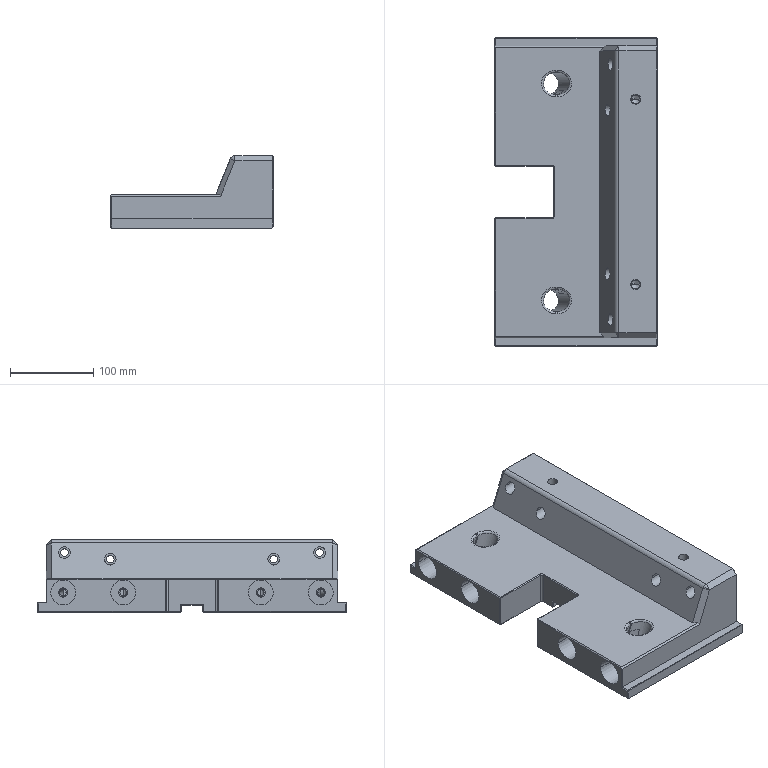Part | Creo | 1 solid | 339 faces | box 195 x 370.009 x 86.7 mm | volume 3296246 mm3 | plane 148 | cylinder 125 | cone 50 | spline 16 | commonest cylinder face diameters 8 x26 1.5 x16 9 x16 17.4 x12 24 x12 14 x8